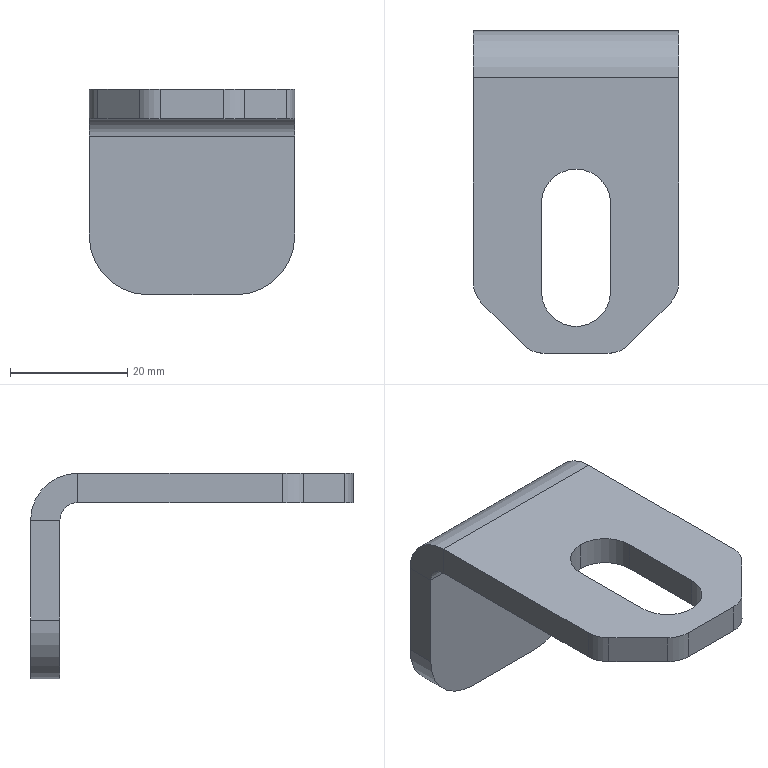Part | SolidWorks | features Fillet 2, Chamfer 1, FlatPattern 1, ICE 1, SMBaseFlange 1, SheetMetal 1 | 1 solid | 27 faces | box 35 x 55 x 35 mm | volume 12305 mm3 | plane 16 | cylinder 11 | commonest cylinder face diameters 10 x4 11.8 x3 20 x2 6 x1 16 x1
STEP:
#1=CARTESIAN_POINT('',(23.4,-29.5,0.));
#2=VERTEX_POINT('',#1);
#3=CARTESIAN_POINT('',(17.5,-23.6,0.));
#4=VERTEX_POINT('',#3);
#5=CARTESIAN_POINT('',(17.5,-29.5,0.));
#6=DIRECTION('',(0.,0.,1.));
#7=DIRECTION('',(0.,1.,0.));
#8=AXIS2_PLACEMENT_3D('',#5,#6,#7);
#9=CIRCLE('',#8,5.9);
#10=EDGE_CURVE('',#2,#4,#9,.T.);
#11=ORIENTED_EDGE('',*,*,#10,.T.);
#12=CARTESIAN_POINT('',(17.5,-23.6,-5.));
#13=VERTEX_POINT('',#12);
#14=CARTESIAN_POINT('',(17.5,-23.6,0.001));
#15=DIRECTION('',(0.,0.,-1.));
#16=VECTOR('',#15,1000.);
#17=LINE('',#14,#16);
#18=EDGE_CURVE('',#4,#13,#17,.T.);
#19=ORIENTED_EDGE('',*,*,#18,.T.);
#20=CARTESIAN_POINT('',(23.4,-29.5,-5.));
#21=VERTEX_POINT('',#20);
#22=CARTESIAN_POINT('',(17.5,-29.5,-5.));
#23=DIRECTION('',(0.,0.,-1.));
#24=DIRECTION('',(0.,1.,0.));
#25=AXIS2_PLACEMENT_3D('',#22,#23,#24);
#26=CIRCLE('',#25,5.9);
#27=EDGE_CURVE('',#13,#21,#26,.T.);
#28=ORIENTED_EDGE('',*,*,#27,.T.);
#29=CARTESIAN_POINT('',(23.4,-29.5,0.001));
#30=DIRECTION('',(0.,0.,-1.));
#31=VECTOR('',#30,1000.);
#32=LINE('',#29,#31);
#33=EDGE_CURVE('',#2,#21,#32,.T.);
#34=ORIENTED_EDGE('',*,*,#33,.F.);
#35=EDGE_LOOP('',(#11,#19,#28,#34));
#36=FACE_OUTER_BOUND('',#35,.T.);
#37=CARTESIAN_POINT('',(17.5,-29.5,0.001));
#38=DIRECTION('',(0.,0.,-1.));
#39=DIRECTION('',(0.,1.,0.));
#40=AXIS2_PLACEMENT_3D('',#37,#38,#39);
#41=CYLINDRICAL_SURFACE('',#40,5.9);
#42=ADVANCED_FACE('',(#36),#41,.F.);
#43=CARTESIAN_POINT('',(35.,0.,-8.));
#44=VERTEX_POINT('',#43);
#45=CARTESIAN_POINT('',(35.,-5.,-8.));
#46=VERTEX_POINT('',#45);
#47=CARTESIAN_POINT('',(35.,0.,-8.));
#48=DIRECTION('',(0.,-1.,0.));
#49=VECTOR('',#48,1000.);
#50=LINE('',#47,#49);
#51=EDGE_CURVE('',#44,#46,#50,.T.);
#52=ORIENTED_EDGE('',*,*,#51,.F.);
#53=CARTESIAN_POINT('',(35.,-8.,0.));
#54=VERTEX_POINT('',#53);
#55=CARTESIAN_POINT('',(35.,-8.,-8.));
#56=DIRECTION('',(1.,0.,0.));
#57=DIRECTION('',(0.,0.,1.));
#58=AXIS2_PLACEMENT_3D('',#55,#56,#57);
#59=CIRCLE('',#58,8.);
#60=EDGE_CURVE('',#44,#54,#59,.T.);
#61=ORIENTED_EDGE('',*,*,#60,.T.);
#62=CARTESIAN_POINT('',(35.,-8.,-5.));
#63=VERTEX_POINT('',#62);
#64=CARTESIAN_POINT('',(35.,-8.,-5.));
#65=DIRECTION('',(0.,0.,1.));
#66=VECTOR('',#65,1000.);
#67=LINE('',#64,#66);
#68=EDGE_CURVE('',#63,#54,#67,.T.);
#69=ORIENTED_EDGE('',*,*,#68,.F.);
#70=CARTESIAN_POINT('',(35.,-8.,-8.));
#71=DIRECTION('',(1.,0.,0.));
#72=DIRECTION('',(0.,0.,-1.));
#73=AXIS2_PLACEMENT_3D('',#70,#71,#72);
#74=CIRCLE('',#73,3.);
#75=EDGE_CURVE('',#46,#63,#74,.T.);
#76=ORIENTED_EDGE('',*,*,#75,.F.);
#77=EDGE_LOOP('',(#52,#61,#69,#76));
#78=FACE_OUTER_BOUND('',#77,.T.);
#79=CARTESIAN_POINT('',(35.,0.,-8.));
#80=DIRECTION('',(1.,0.,0.));
#81=DIRECTION('',(0.,0.,-1.));
#82=AXIS2_PLACEMENT_3D('',#79,#80,#81);
#83=PLANE('',#82);
#84=ADVANCED_FACE('',(#78),#83,.T.);
#85=CARTESIAN_POINT('',(35.,-5.,-25.));
#86=VERTEX_POINT('',#85);
#87=CARTESIAN_POINT('',(35.,-5.,0.));
#88=DIRECTION('',(0.,0.,1.));
#89=VECTOR('',#88,1000.);
#90=LINE('',#87,#89);
#91=EDGE_CURVE('',#86,#46,#90,.T.);
#92=ORIENTED_EDGE('',*,*,#91,.F.);
#93=CARTESIAN_POINT('',(35.,0.,-25.));
#94=VERTEX_POINT('',#93);
#95=CARTESIAN_POINT('',(35.,-8.,-25.));
#96=DIRECTION('',(0.,1.,0.));
#97=VECTOR('',#96,1000.);
#98=LINE('',#95,#97);
#99=EDGE_CURVE('',#86,#94,#98,.T.);
#100=ORIENTED_EDGE('',*,*,#99,.T.);
#101=CARTESIAN_POINT('',(35.,0.,0.));
#102=DIRECTION('',(0.,0.,1.));
#103=VECTOR('',#102,1000.);
#104=LINE('',#101,#103);
#105=EDGE_CURVE('',#94,#44,#104,.T.);
#106=ORIENTED_EDGE('',*,*,#105,.T.);
#107=ORIENTED_EDGE('',*,*,#51,.T.);
#108=EDGE_LOOP('',(#92,#100,#106,#107));
#109=FACE_OUTER_BOUND('',#108,.T.);
#110=CARTESIAN_POINT('',(35.,-8.,-5.));
#111=DIRECTION('',(1.,0.,0.));
#112=DIRECTION('',(0.,0.,-1.));
#113=AXIS2_PLACEMENT_3D('',#110,#111,#112);
#114=PLANE('',#113);
#115=ADVANCED_FACE('',(#109),#114,.T.);
#116=CARTESIAN_POINT('',(0.,-8.,0.));
#117=VERTEX_POINT('',#116);
#118=CARTESIAN_POINT('',(0.,-8.,-5.));
#119=VERTEX_POINT('',#118);
#120=CARTESIAN_POINT('',(0.,-8.,0.));
#121=DIRECTION('',(0.,0.,-1.));
#122=VECTOR('',#121,1000.);
#123=LINE('',#120,#122);
#124=EDGE_CURVE('',#117,#119,#123,.T.);
#125=ORIENTED_EDGE('',*,*,#124,.F.);
#126=CARTESIAN_POINT('',(0.,0.,-8.));
#127=VERTEX_POINT('',#126);
#128=CARTESIAN_POINT('',(0.,-8.,-8.));
#129=DIRECTION('',(1.,0.,0.));
#130=DIRECTION('',(0.,0.,1.));
#131=AXIS2_PLACEMENT_3D('',#128,#129,#130);
#132=CIRCLE('',#131,8.);
#133=EDGE_CURVE('',#127,#117,#132,.T.);
#134=ORIENTED_EDGE('',*,*,#133,.F.);
#135=CARTESIAN_POINT('',(0.,-5.,-8.));
#136=VERTEX_POINT('',#135);
#137=CARTESIAN_POINT('',(0.,-5.,-8.));
#138=DIRECTION('',(0.,1.,0.));
#139=VECTOR('',#138,1000.);
#140=LINE('',#137,#139);
#141=EDGE_CURVE('',#136,#127,#140,.T.);
#142=ORIENTED_EDGE('',*,*,#141,.F.);
#143=CARTESIAN_POINT('',(0.,-8.,-8.));
#144=DIRECTION('',(1.,0.,0.));
#145=DIRECTION('',(0.,0.,-1.));
#146=AXIS2_PLACEMENT_3D('',#143,#144,#145);
#147=CIRCLE('',#146,3.);
#148=EDGE_CURVE('',#136,#119,#147,.T.);
#149=ORIENTED_EDGE('',*,*,#148,.T.);
#150=EDGE_LOOP('',(#125,#134,#142,#149));
#151=FACE_OUTER_BOUND('',#150,.T.);
#152=CARTESIAN_POINT('',(0.,-8.,0.));
#153=DIRECTION('',(-1.,0.,0.));
#154=DIRECTION('',(0.,0.,1.));
#155=AXIS2_PLACEMENT_3D('',#152,#153,#154);
#156=PLANE('',#155);
#157=ADVANCED_FACE('',(#151),#156,.T.);
#158=CARTESIAN_POINT('',(0.,-42.929,-5.));
#159=VERTEX_POINT('',#158);
#160=CARTESIAN_POINT('',(0.,0.,-5.));
#161=DIRECTION('',(0.,-1.,0.));
#162=VECTOR('',#161,1000.);
#163=LINE('',#160,#162);
#164=EDGE_CURVE('',#119,#159,#163,.T.);
#165=ORIENTED_EDGE('',*,*,#164,.T.);
#166=CARTESIAN_POINT('',(0.,-42.929,0.));
#167=VERTEX_POINT('',#166);
#168=CARTESIAN_POINT('',(0.,-42.929,-8.));
#169=DIRECTION('',(0.,0.,1.));
#170=VECTOR('',#169,1000.);
#171=LINE('',#168,#170);
#172=EDGE_CURVE('',#159,#167,#171,.T.);
#173=ORIENTED_EDGE('',*,*,#172,.T.);
#174=CARTESIAN_POINT('',(0.,0.,0.));
#175=DIRECTION('',(0.,-1.,0.));
#176=VECTOR('',#175,1000.);
#177=LINE('',#174,#176);
#178=EDGE_CURVE('',#117,#167,#177,.T.);
#179=ORIENTED_EDGE('',*,*,#178,.F.);
#180=ORIENTED_EDGE('',*,*,#124,.T.);
#181=EDGE_LOOP('',(#165,#173,#179,#180));
#182=FACE_OUTER_BOUND('',#181,.T.);
#183=CARTESIAN_POINT('',(0.,-5.,-8.));
#184=DIRECTION('',(-1.,0.,0.));
#185=DIRECTION('',(0.,0.,1.));
#186=AXIS2_PLACEMENT_3D('',#183,#184,#185);
#187=PLANE('',#186);
#188=ADVANCED_FACE('',(#182),#187,.T.);
#189=CARTESIAN_POINT('',(11.6,-29.5,0.));
#190=VERTEX_POINT('',#189);
#191=CARTESIAN_POINT('',(11.6,-44.5,0.));
#192=VERTEX_POINT('',#191);
#193=CARTESIAN_POINT('',(11.6,-29.5,0.));
#194=DIRECTION('',(0.,-1.,0.));
#195=VECTOR('',#194,1000.);
#196=LINE('',#193,#195);
#197=EDGE_CURVE('',#190,#192,#196,.T.);
#198=ORIENTED_EDGE('',*,*,#197,.F.);
#199=CARTESIAN_POINT('',(17.5,-29.5,0.));
#200=DIRECTION('',(0.,0.,1.));
#201=DIRECTION('',(0.,1.,0.));
#202=AXIS2_PLACEMENT_3D('',#199,#200,#201);
#203=CIRCLE('',#202,5.9);
#204=EDGE_CURVE('',#4,#190,#203,.T.);
#205=ORIENTED_EDGE('',*,*,#204,.F.);
#206=ORIENTED_EDGE('',*,*,#10,.F.);
#207=CARTESIAN_POINT('',(23.4,-44.5,0.));
#208=VERTEX_POINT('',#207);
#209=CARTESIAN_POINT('',(23.4,-29.5,0.));
#210=DIRECTION('',(0.,1.,0.));
#211=VECTOR('',#210,1000.);
#212=LINE('',#209,#211);
#213=EDGE_CURVE('',#208,#2,#212,.T.);
#214=ORIENTED_EDGE('',*,*,#213,.F.);
#215=CARTESIAN_POINT('',(17.5,-44.5,0.));
#216=DIRECTION('',(0.,0.,1.));
#217=DIRECTION('',(0.,1.,0.));
#218=AXIS2_PLACEMENT_3D('',#215,#216,#217);
#219=CIRCLE('',#218,5.9);
#220=EDGE_CURVE('',#192,#208,#219,.T.);
#221=ORIENTED_EDGE('',*,*,#220,.F.);
#222=EDGE_LOOP('',(#198,#205,#206,#214,#221));
#223=FACE_BOUND('',#222,.T.);
#224=CARTESIAN_POINT('',(26.464,-53.536,0.));
#225=VERTEX_POINT('',#224);
#226=CARTESIAN_POINT('',(33.536,-46.464,0.));
#227=VERTEX_POINT('',#226);
#228=CARTESIAN_POINT('',(25.,-55.,0.));
#229=DIRECTION('',(0.7071,0.7071,0.));
#230=VECTOR('',#229,1000.);
#231=LINE('',#228,#230);
#232=EDGE_CURVE('',#225,#227,#231,.T.);
#233=ORIENTED_EDGE('',*,*,#232,.T.);
#234=CARTESIAN_POINT('',(35.,-42.929,0.));
#235=VERTEX_POINT('',#234);
#236=CARTESIAN_POINT('',(30.,-42.929,0.));
#237=DIRECTION('',(0.,0.,1.));
#238=DIRECTION('',(0.,1.,0.));
#239=AXIS2_PLACEMENT_3D('',#236,#237,#238);
#240=CIRCLE('',#239,5.);
#241=EDGE_CURVE('',#227,#235,#240,.T.);
#242=ORIENTED_EDGE('',*,*,#241,.T.);
#243=CARTESIAN_POINT('',(35.,0.,0.));
#244=DIRECTION('',(0.,-1.,0.));
#245=VECTOR('',#244,1000.);
#246=LINE('',#243,#245);
#247=EDGE_CURVE('',#54,#235,#246,.T.);
#248=ORIENTED_EDGE('',*,*,#247,.F.);
#249=CARTESIAN_POINT('',(35.,-8.,0.));
#250=DIRECTION('',(-1.,0.,0.));
#251=VECTOR('',#250,1000.);
#252=LINE('',#249,#251);
#253=EDGE_CURVE('',#54,#117,#252,.T.);
#254=ORIENTED_EDGE('',*,*,#253,.T.);
#255=ORIENTED_EDGE('',*,*,#178,.T.);
#256=CARTESIAN_POINT('',(1.464,-46.464,0.));
#257=VERTEX_POINT('',#256);
#258=CARTESIAN_POINT('',(5.,-42.929,0.));
#259=DIRECTION('',(0.,0.,1.));
#260=DIRECTION('',(0.,1.,0.));
#261=AXIS2_PLACEMENT_3D('',#258,#259,#260);
#262=CIRCLE('',#261,5.);
#263=EDGE_CURVE('',#167,#257,#262,.T.);
#264=ORIENTED_EDGE('',*,*,#263,.T.);
#265=CARTESIAN_POINT('',(8.536,-53.536,0.));
#266=VERTEX_POINT('',#265);
#267=CARTESIAN_POINT('',(0.,-45.,0.));
#268=DIRECTION('',(0.7071,-0.7071,0.));
#269=VECTOR('',#268,1000.);
#270=LINE('',#267,#269);
#271=EDGE_CURVE('',#257,#266,#270,.T.);
#272=ORIENTED_EDGE('',*,*,#271,.T.);
#273=CARTESIAN_POINT('',(12.071,-55.,0.));
#274=VERTEX_POINT('',#273);
#275=CARTESIAN_POINT('',(12.071,-50.,0.));
#276=DIRECTION('',(0.,0.,1.));
#277=DIRECTION('',(0.,1.,0.));
#278=AXIS2_PLACEMENT_3D('',#275,#276,#277);
#279=CIRCLE('',#278,5.);
#280=EDGE_CURVE('',#266,#274,#279,.T.);
#281=ORIENTED_EDGE('',*,*,#280,.T.);
#282=CARTESIAN_POINT('',(22.929,-55.,0.));
#283=VERTEX_POINT('',#282);
#284=CARTESIAN_POINT('',(35.,-55.,0.));
#285=DIRECTION('',(-1.,0.,0.));
#286=VECTOR('',#285,1000.);
#287=LINE('',#284,#286);
#288=EDGE_CURVE('',#283,#274,#287,.T.);
#289=ORIENTED_EDGE('',*,*,#288,.F.);
#290=CARTESIAN_POINT('',(22.929,-50.,0.));
#291=DIRECTION('',(0.,0.,1.));
#292=DIRECTION('',(0.,1.,0.));
#293=AXIS2_PLACEMENT_3D('',#290,#291,#292);
#294=CIRCLE('',#293,5.);
#295=EDGE_CURVE('',#283,#225,#294,.T.);
#296=ORIENTED_EDGE('',*,*,#295,.T.);
#297=EDGE_LOOP('',(#233,#242,#248,#254,#255,#264,#272,#281,#289,#296));
#298=FACE_OUTER_BOUND('',#297,.T.);
#299=CARTESIAN_POINT('',(35.,0.,0.));
#300=DIRECTION('',(0.,0.,-1.));
#301=DIRECTION('',(0.,1.,0.));
#302=AXIS2_PLACEMENT_3D('',#299,#300,#301);
#303=PLANE('',#302);
#304=ADVANCED_FACE('',(#223,#298),#303,.F.);
#305=CARTESIAN_POINT('',(22.929,-55.,-5.));
#306=VERTEX_POINT('',#305);
#307=CARTESIAN_POINT('',(12.071,-55.,-5.));
#308=VERTEX_POINT('',#307);
#309=CARTESIAN_POINT('',(35.,-55.,-5.));
#310=DIRECTION('',(-1.,0.,0.));
#311=VECTOR('',#310,1000.);
#312=LINE('',#309,#311);
#313=EDGE_CURVE('',#306,#308,#312,.T.);
#314=ORIENTED_EDGE('',*,*,#313,.F.);
#315=CARTESIAN_POINT('',(22.929,-55.,-5.));
#316=DIRECTION('',(0.,0.,1.));
#317=VECTOR('',#316,1000.);
#318=LINE('',#315,#317);
#319=EDGE_CURVE('',#306,#283,#318,.T.);
#320=ORIENTED_EDGE('',*,*,#319,.T.);
#321=ORIENTED_EDGE('',*,*,#288,.T.);
#322=CARTESIAN_POINT('',(12.071,-55.,-5.));
#323=DIRECTION('',(0.,0.,-1.));
#324=VECTOR('',#323,1000.);
#325=LINE('',#322,#324);
#326=EDGE_CURVE('',#274,#308,#325,.T.);
#327=ORIENTED_EDGE('',*,*,#326,.T.);
#328=EDGE_LOOP('',(#314,#320,#321,#327));
#329=FACE_OUTER_BOUND('',#328,.T.);
#330=CARTESIAN_POINT('',(35.,-55.,-5.));
#331=DIRECTION('',(0.,-1.,0.));
#332=DIRECTION('',(0.,0.,-1.));
#333=AXIS2_PLACEMENT_3D('',#330,#331,#332);
#334=PLANE('',#333);
#335=ADVANCED_FACE('',(#329),#334,.T.);
#336=CARTESIAN_POINT('',(11.6,-29.5,-5.));
#337=VERTEX_POINT('',#336);
#338=CARTESIAN_POINT('',(17.5,-29.5,-5.));
#339=DIRECTION('',(0.,0.,-1.));
#340=DIRECTION('',(0.,1.,0.));
#341=AXIS2_PLACEMENT_3D('',#338,#339,#340);
#342=CIRCLE('',#341,5.9);
#343=EDGE_CURVE('',#337,#13,#342,.T.);
#344=ORIENTED_EDGE('',*,*,#343,.F.);
#345=CARTESIAN_POINT('',(11.6,-44.5,-5.));
#346=VERTEX_POINT('',#345);
#347=CARTESIAN_POINT('',(11.6,-29.5,-5.));
#348=DIRECTION('',(0.,1.,0.));
#349=VECTOR('',#348,1000.);
#350=LINE('',#347,#349);
#351=EDGE_CURVE('',#346,#337,#350,.T.);
#352=ORIENTED_EDGE('',*,*,#351,.F.);
#353=CARTESIAN_POINT('',(23.4,-44.5,-5.));
#354=VERTEX_POINT('',#353);
#355=CARTESIAN_POINT('',(17.5,-44.5,-5.));
#356=DIRECTION('',(0.,0.,-1.));
#357=DIRECTION('',(0.,1.,0.));
#358=AXIS2_PLACEMENT_3D('',#355,#356,#357);
#359=CIRCLE('',#358,5.9);
#360=EDGE_CURVE('',#354,#346,#359,.T.);
#361=ORIENTED_EDGE('',*,*,#360,.F.);
#362=CARTESIAN_POINT('',(23.4,-29.5,-5.));
#363=DIRECTION('',(0.,-1.,0.));
#364=VECTOR('',#363,1000.);
#365=LINE('',#362,#364);
#366=EDGE_CURVE('',#21,#354,#365,.T.);
#367=ORIENTED_EDGE('',*,*,#366,.F.);
#368=ORIENTED_EDGE('',*,*,#27,.F.);
#369=EDGE_LOOP('',(#344,#352,#361,#367,#368));
#370=FACE_BOUND('',#369,.T.);
#371=CARTESIAN_POINT('',(35.,-42.929,-5.));
#372=VERTEX_POINT('',#371);
#373=CARTESIAN_POINT('',(35.,0.,-5.));
#374=DIRECTION('',(0.,-1.,0.));
#375=VECTOR('',#374,1000.);
#376=LINE('',#373,#375);
#377=EDGE_CURVE('',#63,#372,#376,.T.);
#378=ORIENTED_EDGE('',*,*,#377,.T.);
#379=CARTESIAN_POINT('',(33.536,-46.464,-5.));
#380=VERTEX_POINT('',#379);
#381=CARTESIAN_POINT('',(30.,-42.929,-5.));
#382=DIRECTION('',(0.,0.,-1.));
#383=DIRECTION('',(0.,1.,0.));
#384=AXIS2_PLACEMENT_3D('',#381,#382,#383);
#385=CIRCLE('',#384,5.);
#386=EDGE_CURVE('',#372,#380,#385,.T.);
#387=ORIENTED_EDGE('',*,*,#386,.T.);
#388=CARTESIAN_POINT('',(26.464,-53.536,-5.));
#389=VERTEX_POINT('',#388);
#390=CARTESIAN_POINT('',(57.5,-22.5,-5.));
#391=DIRECTION('',(-0.7071,-0.7071,0.));
#392=VECTOR('',#391,1000.);
#393=LINE('',#390,#392);
#394=EDGE_CURVE('',#380,#389,#393,.T.);
#395=ORIENTED_EDGE('',*,*,#394,.T.);
#396=CARTESIAN_POINT('',(22.929,-50.,-5.));
#397=DIRECTION('',(0.,0.,-1.));
#398=DIRECTION('',(0.,1.,0.));
#399=AXIS2_PLACEMENT_3D('',#396,#397,#398);
#400=CIRCLE('',#399,5.);
#401=EDGE_CURVE('',#389,#306,#400,.T.);
#402=ORIENTED_EDGE('',*,*,#401,.T.);
#403=ORIENTED_EDGE('',*,*,#313,.T.);
#404=CARTESIAN_POINT('',(8.536,-53.536,-5.));
#405=VERTEX_POINT('',#404);
#406=CARTESIAN_POINT('',(12.071,-50.,-5.));
#407=DIRECTION('',(0.,0.,-1.));
#408=DIRECTION('',(0.,1.,0.));
#409=AXIS2_PLACEMENT_3D('',#406,#407,#408);
#410=CIRCLE('',#409,5.);
#411=EDGE_CURVE('',#308,#405,#410,.T.);
#412=ORIENTED_EDGE('',*,*,#411,.T.);
#413=CARTESIAN_POINT('',(1.464,-46.464,-5.));
#414=VERTEX_POINT('',#413);
#415=CARTESIAN_POINT('',(-5.,-40.,-5.));
#416=DIRECTION('',(-0.7071,0.7071,0.));
#417=VECTOR('',#416,1000.);
#418=LINE('',#415,#417);
#419=EDGE_CURVE('',#405,#414,#418,.T.);
#420=ORIENTED_EDGE('',*,*,#419,.T.);
#421=CARTESIAN_POINT('',(5.,-42.929,-5.));
#422=DIRECTION('',(0.,0.,-1.));
#423=DIRECTION('',(0.,1.,0.));
#424=AXIS2_PLACEMENT_3D('',#421,#422,#423);
#425=CIRCLE('',#424,5.);
#426=EDGE_CURVE('',#414,#159,#425,.T.);
#427=ORIENTED_EDGE('',*,*,#426,.T.);
#428=ORIENTED_EDGE('',*,*,#164,.F.);
#429=CARTESIAN_POINT('',(35.,-8.,-5.));
#430=DIRECTION('',(-1.,0.,0.));
#431=VECTOR('',#430,1000.);
#432=LINE('',#429,#431);
#433=EDGE_CURVE('',#63,#119,#432,.T.);
#434=ORIENTED_EDGE('',*,*,#433,.F.);
#435=EDGE_LOOP('',(#378,#387,#395,#402,#403,#412,#420,#427,#428,#434));
#436=FACE_OUTER_BOUND('',#435,.T.);
#437=CARTESIAN_POINT('',(35.,0.,-5.));
#438=DIRECTION('',(0.,0.,-1.));
#439=DIRECTION('',(0.,1.,0.));
#440=AXIS2_PLACEMENT_3D('',#437,#438,#439);
#441=PLANE('',#440);
#442=ADVANCED_FACE('',(#370,#436),#441,.T.);
#443=ORIENTED_EDGE('',*,*,#148,.F.);
#444=CARTESIAN_POINT('',(35.,-5.,-8.));
#445=DIRECTION('',(-1.,0.,0.));
#446=VECTOR('',#445,1000.);
#447=LINE('',#444,#446);
#448=EDGE_CURVE('',#46,#136,#447,.T.);
#449=ORIENTED_EDGE('',*,*,#448,.F.);
#450=ORIENTED_EDGE('',*,*,#75,.T.);
#451=ORIENTED_EDGE('',*,*,#433,.T.);
#452=EDGE_LOOP('',(#443,#449,#450,#451));
#453=FACE_OUTER_BOUND('',#452,.T.);
#454=CARTESIAN_POINT('',(35.,-8.,-8.));
#455=DIRECTION('',(-1.,0.,0.));
#456=DIRECTION('',(0.,0.,1.));
#457=AXIS2_PLACEMENT_3D('',#454,#455,#456);
#458=CYLINDRICAL_SURFACE('',#457,3.);
#459=ADVANCED_FACE('',(#453),#458,.F.);
#460=CARTESIAN_POINT('',(25.,-5.,-35.));
#461=VERTEX_POINT('',#460);
#462=CARTESIAN_POINT('',(10.,-5.,-35.));
#463=VERTEX_POINT('',#462);
#464=CARTESIAN_POINT('',(35.,-5.,-35.));
#465=DIRECTION('',(-1.,0.,0.));
#466=VECTOR('',#465,1000.);
#467=LINE('',#464,#466);
#468=EDGE_CURVE('',#461,#463,#467,.T.);
#469=ORIENTED_EDGE('',*,*,#468,.F.);
#470=CARTESIAN_POINT('',(25.,-5.,-25.));
#471=DIRECTION('',(0.,-1.,0.));
#472=DIRECTION('',(0.,0.,-1.));
#473=AXIS2_PLACEMENT_3D('',#470,#471,#472);
#474=CIRCLE('',#473,10.);
#475=EDGE_CURVE('',#461,#86,#474,.T.);
#476=ORIENTED_EDGE('',*,*,#475,.T.);
#477=ORIENTED_EDGE('',*,*,#91,.T.);
#478=ORIENTED_EDGE('',*,*,#448,.T.);
#479=CARTESIAN_POINT('',(0.,-5.,-25.));
#480=VERTEX_POINT('',#479);
#481=CARTESIAN_POINT('',(0.,-5.,0.));
#482=DIRECTION('',(0.,0.,1.));
#483=VECTOR('',#482,1000.);
#484=LINE('',#481,#483);
#485=EDGE_CURVE('',#480,#136,#484,.T.);
#486=ORIENTED_EDGE('',*,*,#485,.F.);
#487=CARTESIAN_POINT('',(10.,-5.,-25.));
#488=DIRECTION('',(0.,-1.,0.));
#489=DIRECTION('',(0.,0.,-1.));
#490=AXIS2_PLACEMENT_3D('',#487,#488,#489);
#491=CIRCLE('',#490,10.);
#492=EDGE_CURVE('',#480,#463,#491,.T.);
#493=ORIENTED_EDGE('',*,*,#492,.T.);
#494=EDGE_LOOP('',(#469,#476,#477,#478,#486,#493));
#495=FACE_OUTER_BOUND('',#494,.T.);
#496=CARTESIAN_POINT('',(35.,-5.,0.));
#497=DIRECTION('',(0.,-1.,0.));
#498=DIRECTION('',(0.,0.,-1.));
#499=AXIS2_PLACEMENT_3D('',#496,#497,#498);
#500=PLANE('',#499);
#501=ADVANCED_FACE('',(#495),#500,.T.);
#502=CARTESIAN_POINT('',(25.,0.,-35.));
#503=VERTEX_POINT('',#502);
#504=CARTESIAN_POINT('',(10.,0.,-35.));
#505=VERTEX_POINT('',#504);
#506=CARTESIAN_POINT('',(35.,0.,-35.));
#507=DIRECTION('',(-1.,0.,0.));
#508=VECTOR('',#507,1000.);
#509=LINE('',#506,#508);
#510=EDGE_CURVE('',#503,#505,#509,.T.);
#511=ORIENTED_EDGE('',*,*,#510,.F.);
#512=CARTESIAN_POINT('',(25.,0.,-35.));
#513=DIRECTION('',(0.,-1.,0.));
#514=VECTOR('',#513,1000.);
#515=LINE('',#512,#514);
#516=EDGE_CURVE('',#503,#461,#515,.T.);
#517=ORIENTED_EDGE('',*,*,#516,.T.);
#518=ORIENTED_EDGE('',*,*,#468,.T.);
#519=CARTESIAN_POINT('',(10.,0.,-35.));
#520=DIRECTION('',(0.,1.,0.));
#521=VECTOR('',#520,1000.);
#522=LINE('',#519,#521);
#523=EDGE_CURVE('',#463,#505,#522,.T.);
#524=ORIENTED_EDGE('',*,*,#523,.T.);
#525=EDGE_LOOP('',(#511,#517,#518,#524));
#526=FACE_OUTER_BOUND('',#525,.T.);
#527=CARTESIAN_POINT('',(35.,0.,-35.));
#528=DIRECTION('',(0.,0.,-1.));
#529=DIRECTION('',(-1.,0.,0.));
#530=AXIS2_PLACEMENT_3D('',#527,#528,#529);
#531=PLANE('',#530);
#532=ADVANCED_FACE('',(#526),#531,.T.);
#533=ORIENTED_EDGE('',*,*,#105,.F.);
#534=CARTESIAN_POINT('',(25.,0.,-25.));
#535=DIRECTION('',(0.,1.,0.));
#536=DIRECTION('',(0.,0.,-1.));
#537=AXIS2_PLACEMENT_3D('',#534,#535,#536);
#538=CIRCLE('',#537,10.);
#539=EDGE_CURVE('',#94,#503,#538,.T.);
#540=ORIENTED_EDGE('',*,*,#539,.T.);
#541=ORIENTED_EDGE('',*,*,#510,.T.);
#542=CARTESIAN_POINT('',(0.,0.,-25.));
#543=VERTEX_POINT('',#542);
#544=CARTESIAN_POINT('',(10.,0.,-25.));
#545=DIRECTION('',(0.,1.,0.));
#546=DIRECTION('',(0.,0.,-1.));
#547=AXIS2_PLACEMENT_3D('',#544,#545,#546);
#548=CIRCLE('',#547,10.);
#549=EDGE_CURVE('',#505,#543,#548,.T.);
#550=ORIENTED_EDGE('',*,*,#549,.T.);
#551=CARTESIAN_POINT('',(0.,0.,0.));
#552=DIRECTION('',(0.,0.,1.));
#553=VECTOR('',#552,1000.);
#554=LINE('',#551,#553);
#555=EDGE_CURVE('',#543,#127,#554,.T.);
#556=ORIENTED_EDGE('',*,*,#555,.T.);
#557=CARTESIAN_POINT('',(35.,0.,-8.));
#558=DIRECTION('',(-1.,0.,0.));
#559=VECTOR('',#558,1000.);
#560=LINE('',#557,#559);
#561=EDGE_CURVE('',#44,#127,#560,.T.);
#562=ORIENTED_EDGE('',*,*,#561,.F.);
#563=EDGE_LOOP('',(#533,#540,#541,#550,#556,#562));
#564=FACE_OUTER_BOUND('',#563,.T.);
#565=CARTESIAN_POINT('',(35.,0.,0.));
#566=DIRECTION('',(0.,-1.,0.));
#567=DIRECTION('',(0.,0.,-1.));
#568=AXIS2_PLACEMENT_3D('',#565,#566,#567);
#569=PLANE('',#568);
#570=ADVANCED_FACE('',(#564),#569,.F.);
#571=ORIENTED_EDGE('',*,*,#133,.T.);
#572=ORIENTED_EDGE('',*,*,#253,.F.);
#573=ORIENTED_EDGE('',*,*,#60,.F.);
#574=ORIENTED_EDGE('',*,*,#561,.T.);
#575=EDGE_LOOP('',(#571,#572,#573,#574));
#576=FACE_OUTER_BOUND('',#575,.T.);
#577=CARTESIAN_POINT('',(35.,-8.,-8.));
#578=DIRECTION('',(-1.,0.,0.));
#579=DIRECTION('',(0.,0.,1.));
#580=AXIS2_PLACEMENT_3D('',#577,#578,#579);
#581=CYLINDRICAL_SURFACE('',#580,8.);
#582=ADVANCED_FACE('',(#576),#581,.T.);
#583=ORIENTED_EDGE('',*,*,#247,.T.);
#584=CARTESIAN_POINT('',(35.,-42.929,-8.));
#585=DIRECTION('',(0.,0.,-1.));
#586=VECTOR('',#585,1000.);
#587=LINE('',#584,#586);
#588=EDGE_CURVE('',#235,#372,#587,.T.);
#589=ORIENTED_EDGE('',*,*,#588,.T.);
#590=ORIENTED_EDGE('',*,*,#377,.F.);
#591=ORIENTED_EDGE('',*,*,#68,.T.);
#592=EDGE_LOOP('',(#583,#589,#590,#591));
#593=FACE_OUTER_BOUND('',#592,.T.);
#594=CARTESIAN_POINT('',(35.,-8.,-8.));
#595=DIRECTION('',(1.,0.,0.));
#596=DIRECTION('',(0.,0.,-1.));
#597=AXIS2_PLACEMENT_3D('',#594,#595,#596);
#598=PLANE('',#597);
#599=ADVANCED_FACE('',(#593),#598,.T.);
#600=ORIENTED_EDGE('',*,*,#555,.F.);
#601=CARTESIAN_POINT('',(0.,-5.,-25.));
#602=DIRECTION('',(0.,-1.,0.));
#603=VECTOR('',#602,1000.);
#604=LINE('',#601,#603);
#605=EDGE_CURVE('',#543,#480,#604,.T.);
#606=ORIENTED_EDGE('',*,*,#605,.T.);
#607=ORIENTED_EDGE('',*,*,#485,.T.);
#608=ORIENTED_EDGE('',*,*,#141,.T.);
#609=EDGE_LOOP('',(#600,#606,#607,#608));
#610=FACE_OUTER_BOUND('',#609,.T.);
#611=CARTESIAN_POINT('',(0.,-8.,-8.));
#612=DIRECTION('',(1.,0.,0.));
#613=DIRECTION('',(0.,0.,-1.));
#614=AXIS2_PLACEMENT_3D('',#611,#612,#613);
#615=PLANE('',#614);
#616=ADVANCED_FACE('',(#610),#615,.F.);
#617=ORIENTED_EDGE('',*,*,#18,.F.);
#618=ORIENTED_EDGE('',*,*,#204,.T.);
#619=CARTESIAN_POINT('',(11.6,-29.5,0.001));
#620=DIRECTION('',(0.,0.,-1.));
#621=VECTOR('',#620,1000.);
#622=LINE('',#619,#621);
#623=EDGE_CURVE('',#190,#337,#622,.T.);
#624=ORIENTED_EDGE('',*,*,#623,.T.);
#625=ORIENTED_EDGE('',*,*,#343,.T.);
#626=EDGE_LOOP('',(#617,#618,#624,#625));
#627=FACE_OUTER_BOUND('',#626,.T.);
#628=CARTESIAN_POINT('',(17.5,-29.5,0.001));
#629=DIRECTION('',(0.,0.,-1.));
#630=DIRECTION('',(0.,1.,0.));
#631=AXIS2_PLACEMENT_3D('',#628,#629,#630);
#632=CYLINDRICAL_SURFACE('',#631,5.9);
#633=ADVANCED_FACE('',(#627),#632,.F.);
#634=ORIENTED_EDGE('',*,*,#197,.T.);
#635=CARTESIAN_POINT('',(11.6,-44.5,0.001));
#636=DIRECTION('',(0.,0.,-1.));
#637=VECTOR('',#636,1000.);
#638=LINE('',#635,#637);
#639=EDGE_CURVE('',#192,#346,#638,.T.);
#640=ORIENTED_EDGE('',*,*,#639,.T.);
#641=ORIENTED_EDGE('',*,*,#351,.T.);
#642=ORIENTED_EDGE('',*,*,#623,.F.);
#643=EDGE_LOOP('',(#634,#640,#641,#642));
#644=FACE_OUTER_BOUND('',#643,.T.);
#645=CARTESIAN_POINT('',(11.6,-29.5,0.001));
#646=DIRECTION('',(-1.,0.,0.));
#647=DIRECTION('',(0.,0.,1.));
#648=AXIS2_PLACEMENT_3D('',#645,#646,#647);
#649=PLANE('',#648);
#650=ADVANCED_FACE('',(#644),#649,.F.);
#651=ORIENTED_EDGE('',*,*,#220,.T.);
#652=CARTESIAN_POINT('',(23.4,-44.5,0.001));
#653=DIRECTION('',(0.,0.,-1.));
#654=VECTOR('',#653,1000.);
#655=LINE('',#652,#654);
#656=EDGE_CURVE('',#208,#354,#655,.T.);
#657=ORIENTED_EDGE('',*,*,#656,.T.);
#658=ORIENTED_EDGE('',*,*,#360,.T.);
#659=ORIENTED_EDGE('',*,*,#639,.F.);
#660=EDGE_LOOP('',(#651,#657,#658,#659));
#661=FACE_OUTER_BOUND('',#660,.T.);
#662=CARTESIAN_POINT('',(17.5,-44.5,0.001));
#663=DIRECTION('',(0.,0.,-1.));
#664=DIRECTION('',(0.,1.,0.));
#665=AXIS2_PLACEMENT_3D('',#662,#663,#664);
#666=CYLINDRICAL_SURFACE('',#665,5.9);
#667=ADVANCED_FACE('',(#661),#666,.F.);
#668=ORIENTED_EDGE('',*,*,#213,.T.);
#669=ORIENTED_EDGE('',*,*,#33,.T.);
#670=ORIENTED_EDGE('',*,*,#366,.T.);
#671=ORIENTED_EDGE('',*,*,#656,.F.);
#672=EDGE_LOOP('',(#668,#669,#670,#671));
#673=FACE_OUTER_BOUND('',#672,.T.);
#674=CARTESIAN_POINT('',(23.4,-29.5,0.001));
#675=DIRECTION('',(1.,0.,0.));
#676=DIRECTION('',(0.,1.,0.));
#677=AXIS2_PLACEMENT_3D('',#674,#675,#676);
#678=PLANE('',#677);
#679=ADVANCED_FACE('',(#673),#678,.F.);
#680=ORIENTED_EDGE('',*,*,#539,.F.);
#681=ORIENTED_EDGE('',*,*,#99,.F.);
#682=ORIENTED_EDGE('',*,*,#475,.F.);
#683=ORIENTED_EDGE('',*,*,#516,.F.);
#684=EDGE_LOOP('',(#680,#681,#682,#683));
#685=FACE_OUTER_BOUND('',#684,.T.);
#686=CARTESIAN_POINT('',(25.,0.,-25.));
#687=DIRECTION('',(0.,-1.,0.));
#688=DIRECTION('',(0.,0.,-1.));
#689=AXIS2_PLACEMENT_3D('',#686,#687,#688);
#690=CYLINDRICAL_SURFACE('',#689,10.);
#691=ADVANCED_FACE('',(#685),#690,.T.);
#692=ORIENTED_EDGE('',*,*,#549,.F.);
#693=ORIENTED_EDGE('',*,*,#523,.F.);
#694=ORIENTED_EDGE('',*,*,#492,.F.);
#695=ORIENTED_EDGE('',*,*,#605,.F.);
#696=EDGE_LOOP('',(#692,#693,#694,#695));
#697=FACE_OUTER_BOUND('',#696,.T.);
#698=CARTESIAN_POINT('',(10.,-8.,-25.));
#699=DIRECTION('',(0.,1.,0.));
#700=DIRECTION('',(0.,0.,1.));
#701=AXIS2_PLACEMENT_3D('',#698,#699,#700);
#702=CYLINDRICAL_SURFACE('',#701,10.);
#703=ADVANCED_FACE('',(#697),#702,.T.);
#704=ORIENTED_EDGE('',*,*,#394,.F.);
#705=CARTESIAN_POINT('',(33.536,-46.464,-5.));
#706=DIRECTION('',(0.,0.,1.));
#707=VECTOR('',#706,1000.);
#708=LINE('',#705,#707);
#709=EDGE_CURVE('',#380,#227,#708,.T.);
#710=ORIENTED_EDGE('',*,*,#709,.T.);
#711=ORIENTED_EDGE('',*,*,#232,.F.);
#712=CARTESIAN_POINT('',(26.464,-53.536,-5.));
#713=DIRECTION('',(0.,0.,-1.));
#714=VECTOR('',#713,1000.);
#715=LINE('',#712,#714);
#716=EDGE_CURVE('',#225,#389,#715,.T.);
#717=ORIENTED_EDGE('',*,*,#716,.T.);
#718=EDGE_LOOP('',(#704,#710,#711,#717));
#719=FACE_OUTER_BOUND('',#718,.T.);
#720=CARTESIAN_POINT('',(25.,-55.,-5.));
#721=DIRECTION('',(-0.7071,0.7071,0.));
#722=DIRECTION('',(0.,0.,1.));
#723=AXIS2_PLACEMENT_3D('',#720,#721,#722);
#724=PLANE('',#723);
#725=ADVANCED_FACE('',(#719),#724,.F.);
#726=ORIENTED_EDGE('',*,*,#419,.F.);
#727=CARTESIAN_POINT('',(8.536,-53.536,-8.));
#728=DIRECTION('',(0.,0.,1.));
#729=VECTOR('',#728,1000.);
#730=LINE('',#727,#729);
#731=EDGE_CURVE('',#405,#266,#730,.T.);
#732=ORIENTED_EDGE('',*,*,#731,.T.);
#733=ORIENTED_EDGE('',*,*,#271,.F.);
#734=CARTESIAN_POINT('',(1.464,-46.464,-8.));
#735=DIRECTION('',(0.,0.,-1.));
#736=VECTOR('',#735,1000.);
#737=LINE('',#734,#736);
#738=EDGE_CURVE('',#257,#414,#737,.T.);
#739=ORIENTED_EDGE('',*,*,#738,.T.);
#740=EDGE_LOOP('',(#726,#732,#733,#739));
#741=FACE_OUTER_BOUND('',#740,.T.);
#742=CARTESIAN_POINT('',(0.,-45.,-8.));
#743=DIRECTION('',(0.7071,0.7071,0.));
#744=DIRECTION('',(0.,0.,1.));
#745=AXIS2_PLACEMENT_3D('',#742,#743,#744);
#746=PLANE('',#745);
#747=ADVANCED_FACE('',(#741),#746,.F.);
#748=ORIENTED_EDGE('',*,*,#241,.F.);
#749=ORIENTED_EDGE('',*,*,#709,.F.);
#750=ORIENTED_EDGE('',*,*,#386,.F.);
#751=ORIENTED_EDGE('',*,*,#588,.F.);
#752=EDGE_LOOP('',(#748,#749,#750,#751));
#753=FACE_OUTER_BOUND('',#752,.T.);
#754=CARTESIAN_POINT('',(30.,-42.929,-8.));
#755=DIRECTION('',(0.,0.,1.));
#756=DIRECTION('',(1.,0.,0.));
#757=AXIS2_PLACEMENT_3D('',#754,#755,#756);
#758=CYLINDRICAL_SURFACE('',#757,5.);
#759=ADVANCED_FACE('',(#753),#758,.T.);
#760=ORIENTED_EDGE('',*,*,#401,.F.);
#761=ORIENTED_EDGE('',*,*,#716,.F.);
#762=ORIENTED_EDGE('',*,*,#295,.F.);
#763=ORIENTED_EDGE('',*,*,#319,.F.);
#764=EDGE_LOOP('',(#760,#761,#762,#763));
#765=FACE_OUTER_BOUND('',#764,.T.);
#766=CARTESIAN_POINT('',(22.929,-50.,-5.));
#767=DIRECTION('',(0.,0.,-1.));
#768=DIRECTION('',(-1.,0.,0.));
#769=AXIS2_PLACEMENT_3D('',#766,#767,#768);
#770=CYLINDRICAL_SURFACE('',#769,5.);
#771=ADVANCED_FACE('',(#765),#770,.T.);
#772=ORIENTED_EDGE('',*,*,#280,.F.);
#773=ORIENTED_EDGE('',*,*,#731,.F.);
#774=ORIENTED_EDGE('',*,*,#411,.F.);
#775=ORIENTED_EDGE('',*,*,#326,.F.);
#776=EDGE_LOOP('',(#772,#773,#774,#775));
#777=FACE_OUTER_BOUND('',#776,.T.);
#778=CARTESIAN_POINT('',(12.071,-50.,-5.));
#779=DIRECTION('',(0.,0.,1.));
#780=DIRECTION('',(1.,0.,0.));
#781=AXIS2_PLACEMENT_3D('',#778,#779,#780);
#782=CYLINDRICAL_SURFACE('',#781,5.);
#783=ADVANCED_FACE('',(#777),#782,.T.);
#784=ORIENTED_EDGE('',*,*,#426,.F.);
#785=ORIENTED_EDGE('',*,*,#738,.F.);
#786=ORIENTED_EDGE('',*,*,#263,.F.);
#787=ORIENTED_EDGE('',*,*,#172,.F.);
#788=EDGE_LOOP('',(#784,#785,#786,#787));
#789=FACE_OUTER_BOUND('',#788,.T.);
#790=CARTESIAN_POINT('',(5.,-42.929,-8.));
#791=DIRECTION('',(0.,0.,-1.));
#792=DIRECTION('',(-1.,0.,0.));
#793=AXIS2_PLACEMENT_3D('',#790,#791,#792);
#794=CYLINDRICAL_SURFACE('',#793,5.);
#795=ADVANCED_FACE('',(#789),#794,.T.);
#796=CLOSED_SHELL('',(#42,#84,#115,#157,#188,#304,#335,#442,#459,#501,#532,#570,#582,#599,#616,#633,#650,#667,#679,#691,#703,#725,#747,#759,#771,#783,#795));
#797=MANIFOLD_SOLID_BREP('',#796);
#798=CARTESIAN_POINT('',(0.,0.,0.));
#799=DIRECTION('',(0.,0.,1.));
#800=DIRECTION('',(1.,0.,0.));
#801=AXIS2_PLACEMENT_3D('',#798,#799,#800);
#802=(LENGTH_UNIT()NAMED_UNIT(*)SI_UNIT(.MILLI.,.METRE.));
#803=UNCERTAINTY_MEASURE_WITH_UNIT(LENGTH_MEASURE(0.00001),#802,'','');
#804=(NAMED_UNIT(*)PLANE_ANGLE_UNIT()SI_UNIT($,.RADIAN.));
#805=(NAMED_UNIT(*)SI_UNIT($,.STERADIAN.)SOLID_ANGLE_UNIT());
#806=(GEOMETRIC_REPRESENTATION_CONTEXT(3)GLOBAL_UNCERTAINTY_ASSIGNED_CONTEXT((#803))GLOBAL_UNIT_ASSIGNED_CONTEXT((#802,#804,#805))REPRESENTATION_CONTEXT('',''));
#807=ADVANCED_BREP_SHAPE_REPRESENTATION('',(#797,#801),#806);